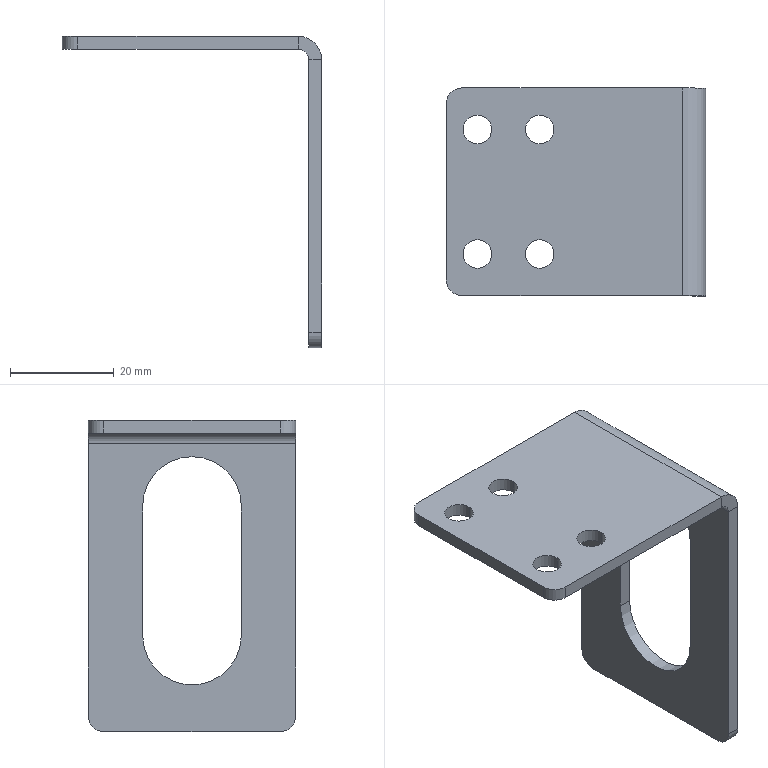Part | STEP file | 1 solid | 31 faces | box 50 x 40 x 60 mm | volume 8457 mm3 | cylinder 17 | plane 14 | commonest cylinder face diameters 5.5 x8 6 x4 19 x3 4 x1 9 x1